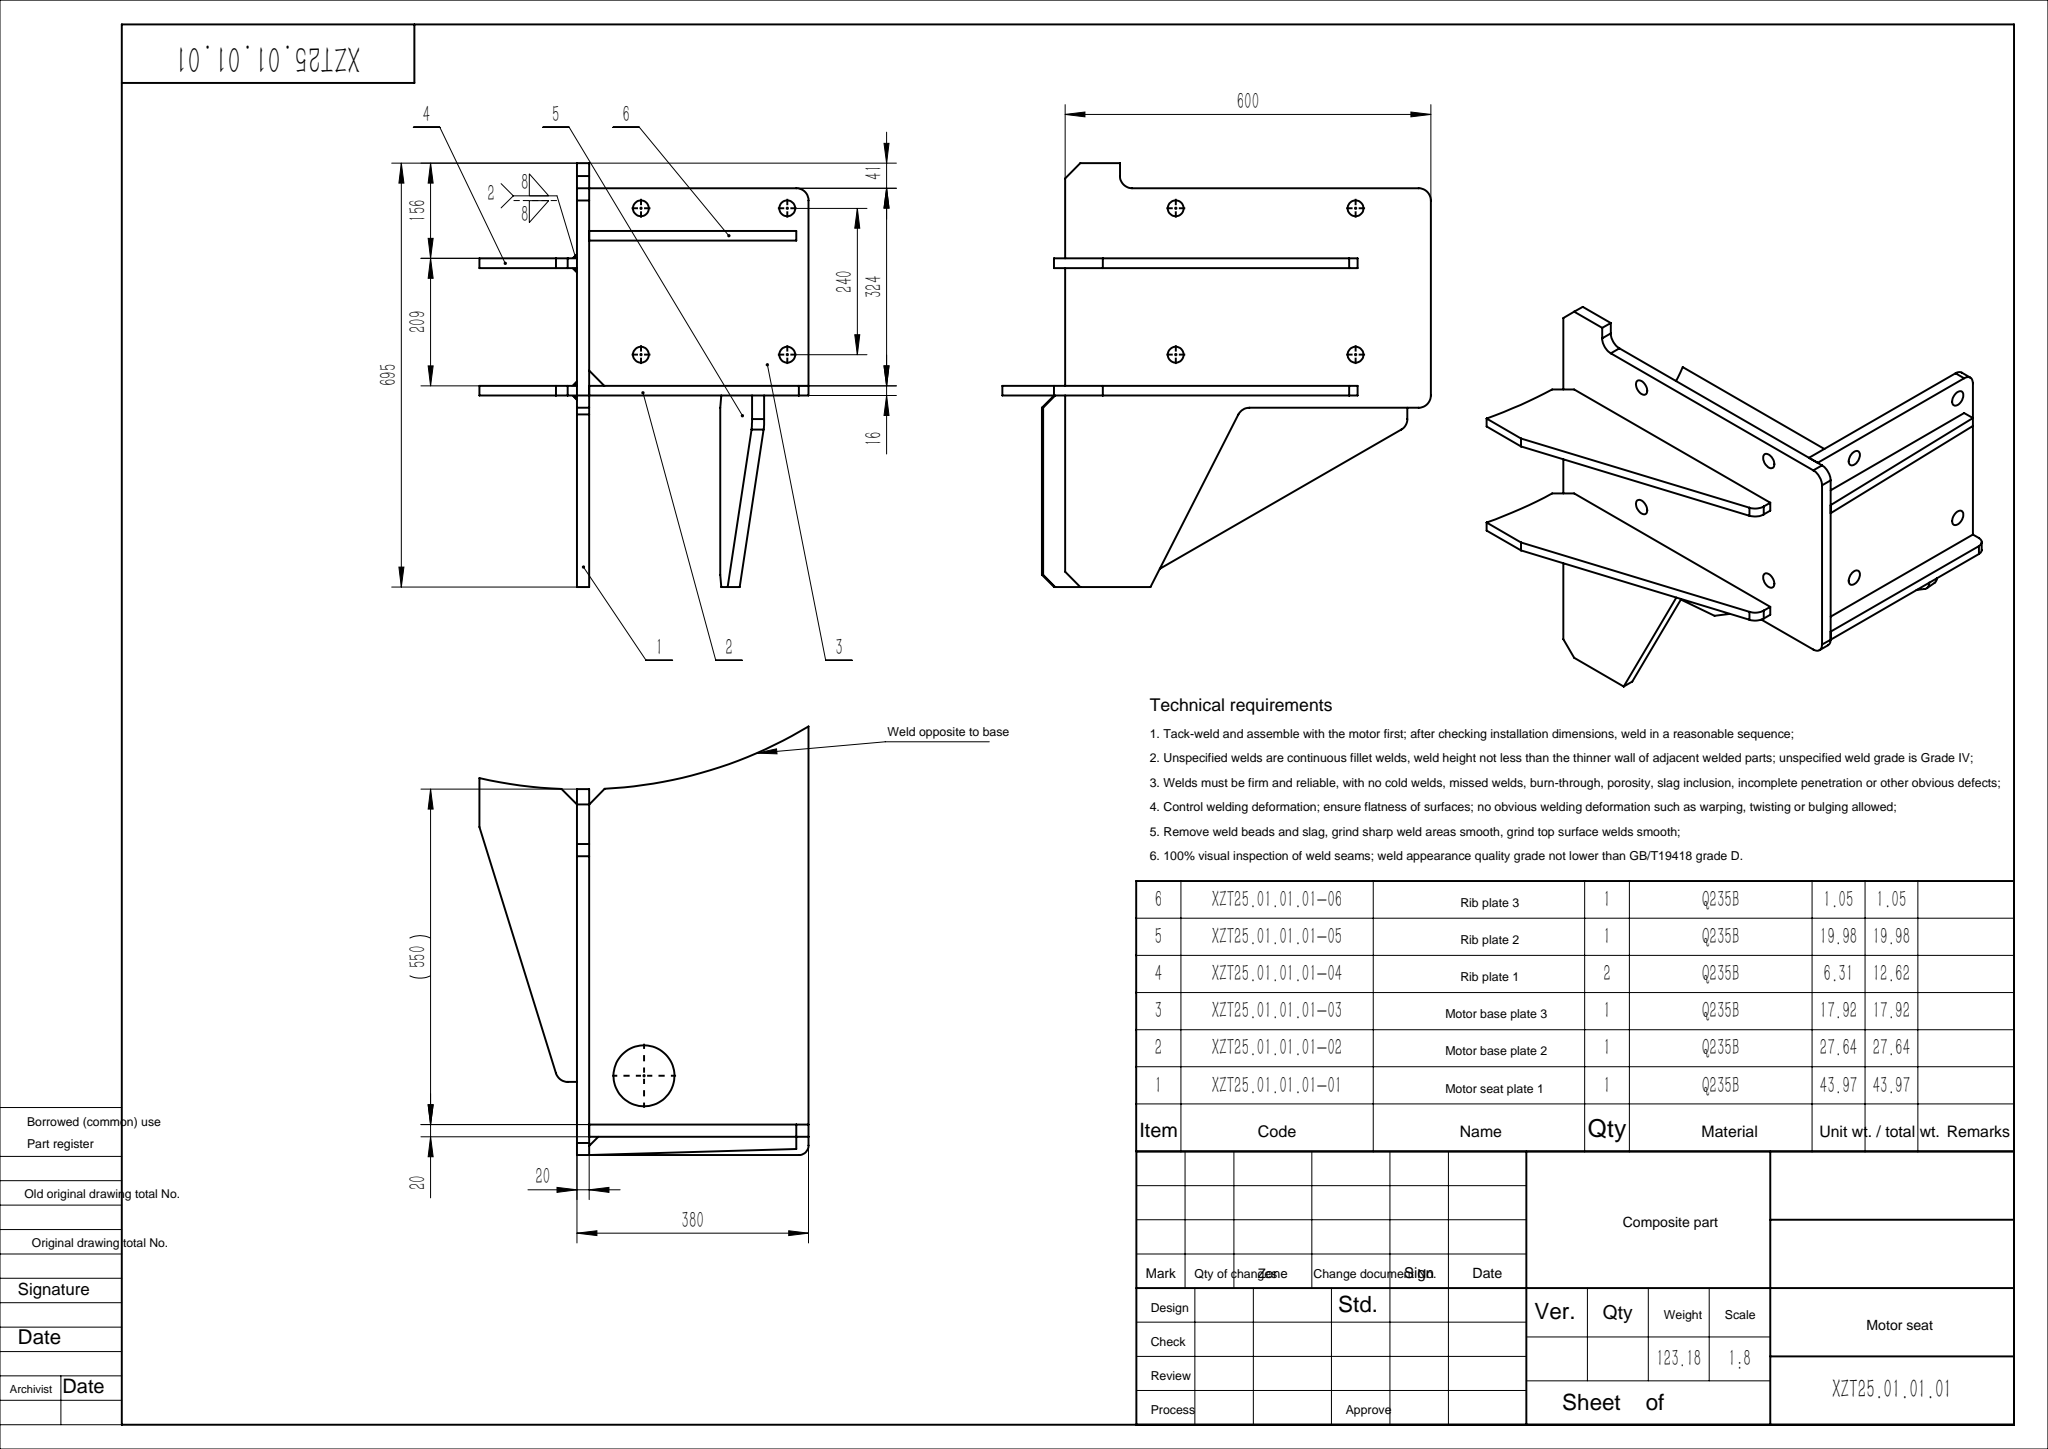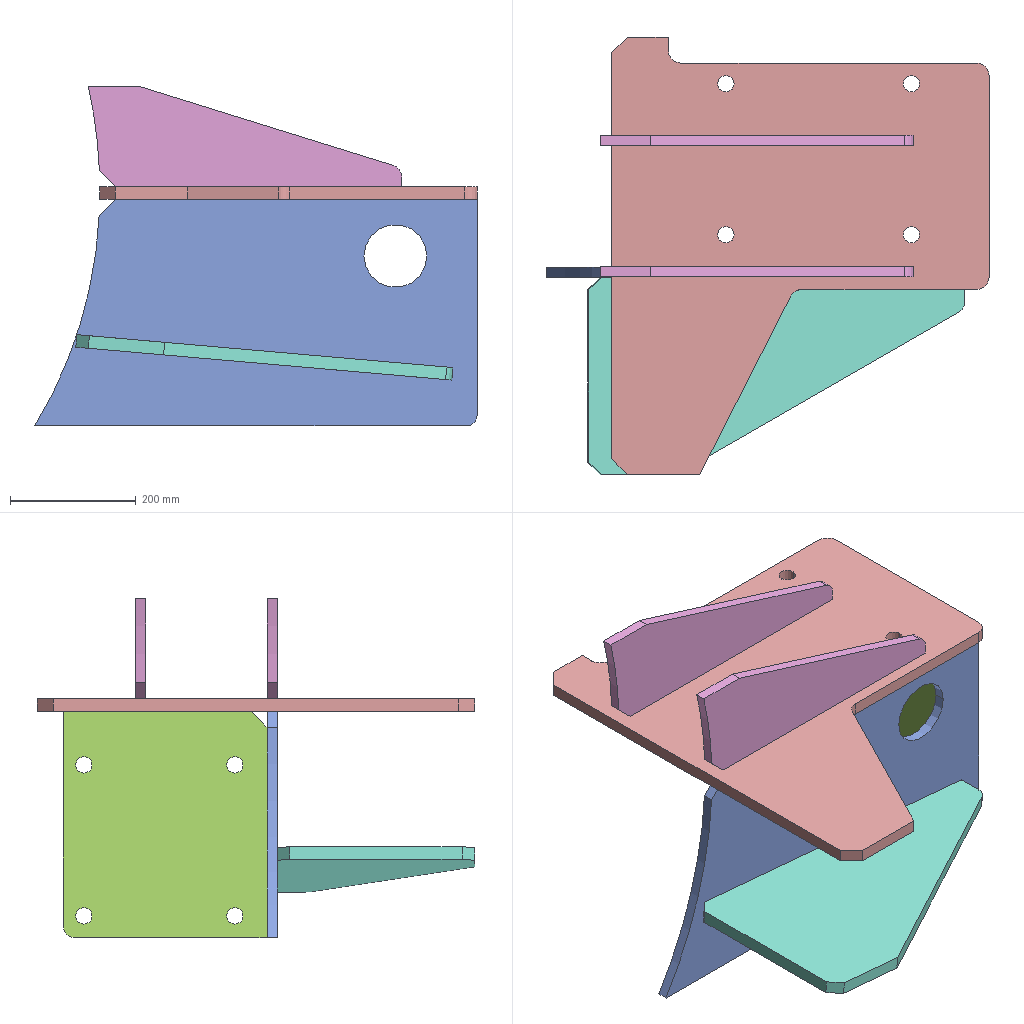Assembly | SolidWorks | 6 different items | 7 placed | box 703 x 695 x 540 mm
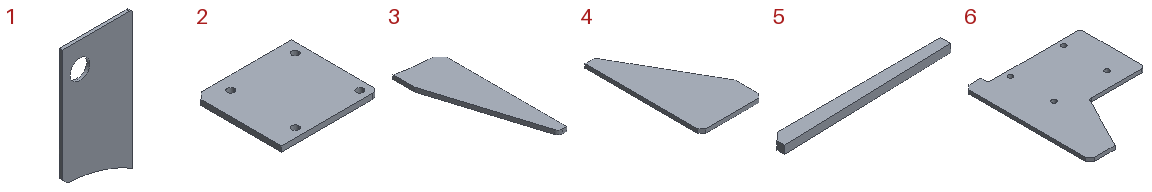Parts list (item | quantity | size | volume | features):
1 | x1 | 360 x 16 x 703 mm | 3520829 mm3 | features Chamfer 1, Extrusion 1, Fillet 1
2 | x1 | 360 x 324 x 20 mm | 2282359 mm3 | features Chamfer 1, Extrusion 1, Fillet 1, HoleWzd 1
3 | x2 | 160 x 498.158 x 16 mm | 803620 mm3 | features Chamfer 1, Extrusion 1, Fillet 1
4 | x1 | 314 x 600 x 20 mm | 2545167 mm3 | features Chamfer 1, Extrusion 1, Fillet 1
5 | x1 | 340 x 30 x 16 mm | 134200 mm3 | features Chamfer 1, Extrusion 1
6 | x1 | 600 x 695 x 20 mm | 5601812 mm3 | features Chamfer 1, Extrusion 1, Fillet 1, HoleWzd 1
Mates (type | each side: item.copy, entity, surface, feature):
Coincident | 6.1 face plane Boss-Extrude1 | 2.1 face plane Boss-Extrude1 | 2 times
Coincident | 2.1 face plane Boss-Extrude1 | 5.1 face plane Boss-Extrude1
Coincident | 6.1 face plane Boss-Extrude1 | 5.1 face plane Boss-Extrude1
Coincident | 6.1 face plane Boss-Extrude1 | 5.1 edge
DistanceDim | 5.1 face plane Boss-Extrude1 | 2.1 face plane Boss-Extrude1
Coincident | 1.1 face plane Boss-Extrude1 | 2.1 face plane Boss-Extrude1
Coincident | 6.1 face plane Boss-Extrude1 | 1.1 face plane Boss-Extrude1 | 2 times
Coincident | 1.1 face plane Boss-Extrude1 | 4.1 face plane Boss-Extrude1
Coincident | 6.1 face plane Boss-Extrude1 | 3.1 face plane Boss-Extrude1
Coincident | 6.1 face plane Boss-Extrude1 | 3.2 face plane Boss-Extrude1
DistanceDim | 3.2 face plane Boss-Extrude1 | 3.1 face plane Boss-Extrude1
Coincident | 3.1 face plane Boss-Extrude1 | 3.2 face plane Boss-Extrude1
Coincident | 1.1 face plane Boss-Extrude1 | 3.2 face plane Boss-Extrude1
DistanceDim | 3.1 face plane Boss-Extrude1 | 6.1 face plane Boss-Extrude1
PlanarAngleDim | 4.1 face plane Boss-Extrude1 | 6.1 face plane Boss-Extrude1
DistanceDim | 4.1 edge | 6.1 face plane Boss-Extrude1
Coincident | 1.1 face cylinder Boss-Extrude1 | 4.1 edge